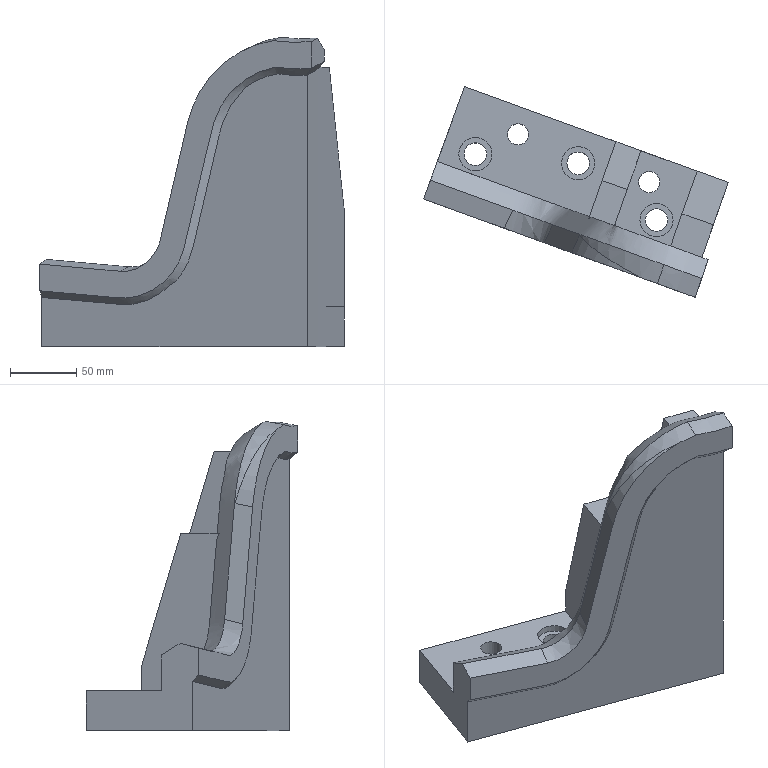Part | NX | features solid 2 | 1 solid | 39 faces | box 229.163 x 158.918 x 232.613 mm | volume 1425987 mm3 | spline 17 | plane 14 | cylinder 8 | commonest cylinder face diameters 17 x3 25 x3 16 x2